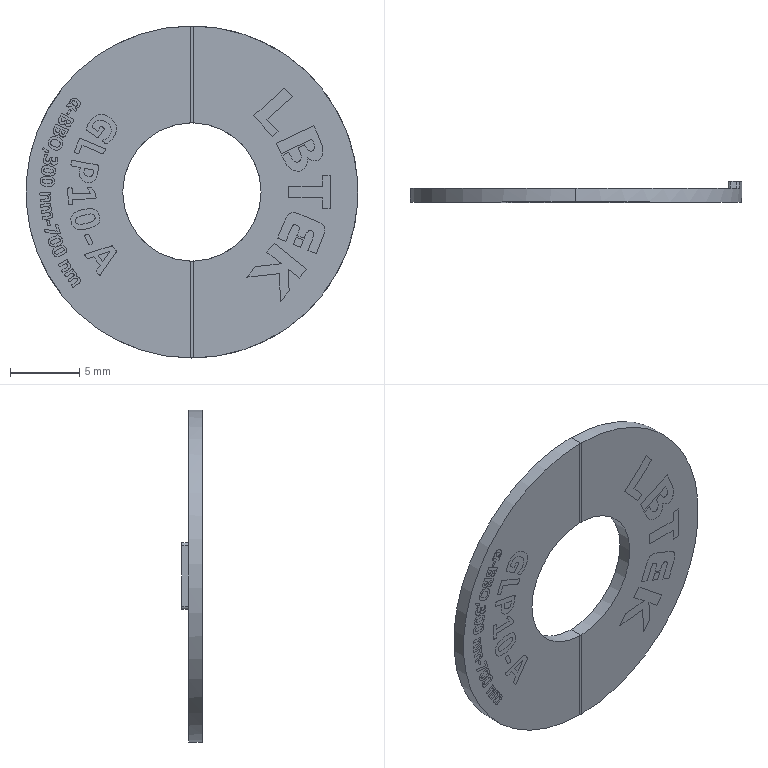Part | STEP file | 1 solid | 64 faces | box 24 x 1.5 x 24 mm | volume 376.014 mm3 | plane 56 | cylinder 8 | commonest cylinder face diameters 0.4 x4 10 x2 24 x2